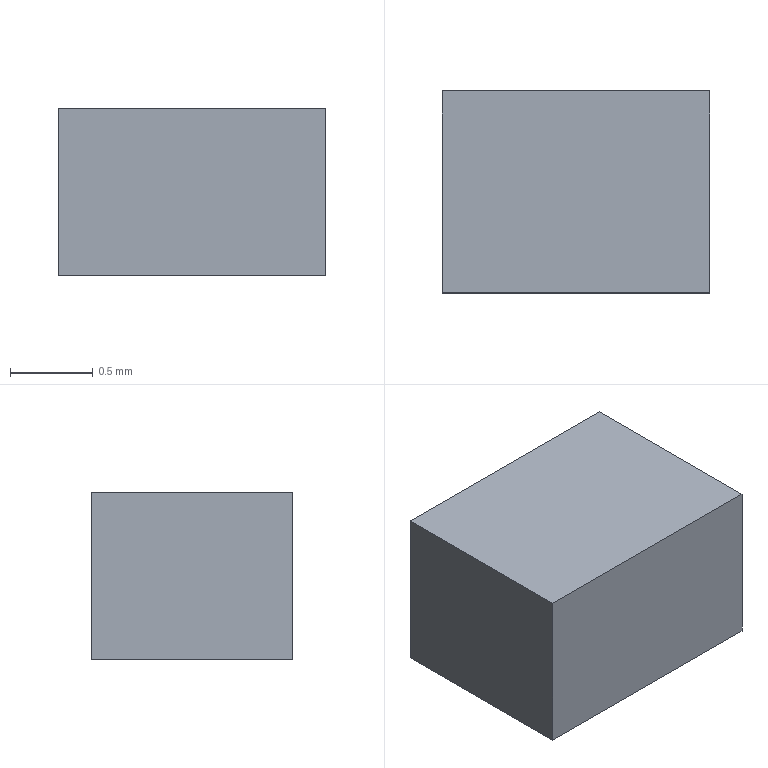Part | Creo | 1 solid | 6 faces | box 1.616 x 1.219 x 1.012 mm | volume 1.993 mm3 | plane 6
STEP:
#1=CARTESIAN_POINT('',(0.,0.,0.));
#2=DIRECTION('',(0.,0.,1.));
#3=DIRECTION('',(1.,0.,0.));
#4=AXIS2_PLACEMENT_3D('',#1,#2,#3);
#5=CARTESIAN_POINT('',(-0.8405,-0.644,0.));
#6=VERTEX_POINT('',#5);
#7=CARTESIAN_POINT('',(0.775,-0.644,0.));
#8=VERTEX_POINT('',#7);
#9=CARTESIAN_POINT('',(-0.8405,-0.644,0.));
#10=DIRECTION('',(1.,0.,0.));
#11=VECTOR('',#10,1.616);
#12=LINE('',#9,#11);
#13=EDGE_CURVE('',#6,#8,#12,.T.);
#14=ORIENTED_EDGE('',*,*,#13,.T.);
#15=CARTESIAN_POINT('',(0.775,0.575,0.));
#16=VERTEX_POINT('',#15);
#17=CARTESIAN_POINT('',(0.775,-0.644,0.));
#18=DIRECTION('',(0.,1.,0.));
#19=VECTOR('',#18,1.219);
#20=LINE('',#17,#19);
#21=EDGE_CURVE('',#8,#16,#20,.T.);
#22=ORIENTED_EDGE('',*,*,#21,.T.);
#23=CARTESIAN_POINT('',(-0.8405,0.575,0.));
#24=VERTEX_POINT('',#23);
#25=CARTESIAN_POINT('',(0.775,0.575,0.));
#26=DIRECTION('',(-1.,0.,0.));
#27=VECTOR('',#26,1.616);
#28=LINE('',#25,#27);
#29=EDGE_CURVE('',#16,#24,#28,.T.);
#30=ORIENTED_EDGE('',*,*,#29,.T.);
#31=CARTESIAN_POINT('',(-0.8405,0.575,0.));
#32=DIRECTION('',(0.,-1.,0.));
#33=VECTOR('',#32,1.219);
#34=LINE('',#31,#33);
#35=EDGE_CURVE('',#24,#6,#34,.T.);
#36=ORIENTED_EDGE('',*,*,#35,.T.);
#37=EDGE_LOOP('',(#14,#22,#30,#36));
#38=FACE_OUTER_BOUND('',#37,.F.);
#39=CARTESIAN_POINT('',(0.,0.,0.));
#40=DIRECTION('',(0.,0.,1.));
#41=DIRECTION('',(1.,0.,0.));
#42=AXIS2_PLACEMENT_3D('',#39,#40,#41);
#43=PLANE('',#42);
#44=ADVANCED_FACE('',(#38),#43,.F.);
#45=ORIENTED_EDGE('',*,*,#13,.F.);
#46=CARTESIAN_POINT('',(-0.8405,-0.644,1.012));
#47=VERTEX_POINT('',#46);
#48=CARTESIAN_POINT('',(-0.8405,-0.644,0.));
#49=DIRECTION('',(0.,0.,1.));
#50=VECTOR('',#49,1.012);
#51=LINE('',#48,#50);
#52=EDGE_CURVE('',#6,#47,#51,.T.);
#53=ORIENTED_EDGE('',*,*,#52,.T.);
#54=CARTESIAN_POINT('',(0.775,-0.644,1.012));
#55=VERTEX_POINT('',#54);
#56=CARTESIAN_POINT('',(-0.8405,-0.644,1.012));
#57=DIRECTION('',(1.,0.,0.));
#58=VECTOR('',#57,1.616);
#59=LINE('',#56,#58);
#60=EDGE_CURVE('',#47,#55,#59,.T.);
#61=ORIENTED_EDGE('',*,*,#60,.T.);
#62=CARTESIAN_POINT('',(0.775,-0.644,0.));
#63=DIRECTION('',(0.,0.,1.));
#64=VECTOR('',#63,1.012);
#65=LINE('',#62,#64);
#66=EDGE_CURVE('',#8,#55,#65,.T.);
#67=ORIENTED_EDGE('',*,*,#66,.F.);
#68=EDGE_LOOP('',(#45,#53,#61,#67));
#69=FACE_OUTER_BOUND('',#68,.F.);
#70=CARTESIAN_POINT('',(-0.8405,-0.644,0.));
#71=DIRECTION('',(0.,-1.,0.));
#72=DIRECTION('',(1.,0.,0.));
#73=AXIS2_PLACEMENT_3D('',#70,#71,#72);
#74=PLANE('',#73);
#75=ADVANCED_FACE('',(#69),#74,.T.);
#76=ORIENTED_EDGE('',*,*,#35,.F.);
#77=CARTESIAN_POINT('',(-0.8405,0.575,1.012));
#78=VERTEX_POINT('',#77);
#79=CARTESIAN_POINT('',(-0.8405,0.575,0.));
#80=DIRECTION('',(0.,0.,1.));
#81=VECTOR('',#80,1.012);
#82=LINE('',#79,#81);
#83=EDGE_CURVE('',#24,#78,#82,.T.);
#84=ORIENTED_EDGE('',*,*,#83,.T.);
#85=CARTESIAN_POINT('',(-0.8405,0.575,1.012));
#86=DIRECTION('',(0.,-1.,0.));
#87=VECTOR('',#86,1.219);
#88=LINE('',#85,#87);
#89=EDGE_CURVE('',#78,#47,#88,.T.);
#90=ORIENTED_EDGE('',*,*,#89,.T.);
#91=ORIENTED_EDGE('',*,*,#52,.F.);
#92=EDGE_LOOP('',(#76,#84,#90,#91));
#93=FACE_OUTER_BOUND('',#92,.F.);
#94=CARTESIAN_POINT('',(-0.8405,0.575,0.));
#95=DIRECTION('',(-1.,0.,0.));
#96=DIRECTION('',(0.,-1.,0.));
#97=AXIS2_PLACEMENT_3D('',#94,#95,#96);
#98=PLANE('',#97);
#99=ADVANCED_FACE('',(#93),#98,.T.);
#100=ORIENTED_EDGE('',*,*,#29,.F.);
#101=CARTESIAN_POINT('',(0.775,0.575,1.012));
#102=VERTEX_POINT('',#101);
#103=CARTESIAN_POINT('',(0.775,0.575,0.));
#104=DIRECTION('',(0.,0.,1.));
#105=VECTOR('',#104,1.012);
#106=LINE('',#103,#105);
#107=EDGE_CURVE('',#16,#102,#106,.T.);
#108=ORIENTED_EDGE('',*,*,#107,.T.);
#109=CARTESIAN_POINT('',(0.775,0.575,1.012));
#110=DIRECTION('',(-1.,0.,0.));
#111=VECTOR('',#110,1.616);
#112=LINE('',#109,#111);
#113=EDGE_CURVE('',#102,#78,#112,.T.);
#114=ORIENTED_EDGE('',*,*,#113,.T.);
#115=ORIENTED_EDGE('',*,*,#83,.F.);
#116=EDGE_LOOP('',(#100,#108,#114,#115));
#117=FACE_OUTER_BOUND('',#116,.F.);
#118=CARTESIAN_POINT('',(0.775,0.575,0.));
#119=DIRECTION('',(0.,1.,0.));
#120=DIRECTION('',(-1.,0.,0.));
#121=AXIS2_PLACEMENT_3D('',#118,#119,#120);
#122=PLANE('',#121);
#123=ADVANCED_FACE('',(#117),#122,.T.);
#124=ORIENTED_EDGE('',*,*,#21,.F.);
#125=ORIENTED_EDGE('',*,*,#66,.T.);
#126=CARTESIAN_POINT('',(0.775,-0.644,1.012));
#127=DIRECTION('',(0.,1.,0.));
#128=VECTOR('',#127,1.219);
#129=LINE('',#126,#128);
#130=EDGE_CURVE('',#55,#102,#129,.T.);
#131=ORIENTED_EDGE('',*,*,#130,.T.);
#132=ORIENTED_EDGE('',*,*,#107,.F.);
#133=EDGE_LOOP('',(#124,#125,#131,#132));
#134=FACE_OUTER_BOUND('',#133,.F.);
#135=CARTESIAN_POINT('',(0.775,-0.644,0.));
#136=DIRECTION('',(1.,0.,0.));
#137=DIRECTION('',(0.,1.,0.));
#138=AXIS2_PLACEMENT_3D('',#135,#136,#137);
#139=PLANE('',#138);
#140=ADVANCED_FACE('',(#134),#139,.T.);
#141=ORIENTED_EDGE('',*,*,#60,.F.);
#142=ORIENTED_EDGE('',*,*,#89,.F.);
#143=ORIENTED_EDGE('',*,*,#113,.F.);
#144=ORIENTED_EDGE('',*,*,#130,.F.);
#145=EDGE_LOOP('',(#141,#142,#143,#144));
#146=FACE_OUTER_BOUND('',#145,.F.);
#147=CARTESIAN_POINT('',(0.,0.,1.012));
#148=DIRECTION('',(0.,0.,1.));
#149=DIRECTION('',(1.,0.,0.));
#150=AXIS2_PLACEMENT_3D('',#147,#148,#149);
#151=PLANE('',#150);
#152=ADVANCED_FACE('',(#146),#151,.T.);
#153=CLOSED_SHELL('',(#44,#75,#99,#123,#140,#152));
#154=MANIFOLD_SOLID_BREP('',#153);
#155=(LENGTH_UNIT()NAMED_UNIT(*)SI_UNIT(.MILLI.,.METRE.));
#156=UNCERTAINTY_MEASURE_WITH_UNIT(LENGTH_MEASURE(0.0002263),#155,'','');
#157=(NAMED_UNIT(*)PLANE_ANGLE_UNIT()SI_UNIT($,.RADIAN.));
#158=PLANE_ANGLE_MEASURE_WITH_UNIT(PLANE_ANGLE_MEASURE(0.01745),#157);
#159=(CONVERSION_BASED_UNIT('DEGREE',#158)NAMED_UNIT(*)PLANE_ANGLE_UNIT());
#160=(NAMED_UNIT(*)SI_UNIT($,.STERADIAN.)SOLID_ANGLE_UNIT());
#161=(GEOMETRIC_REPRESENTATION_CONTEXT(3)GLOBAL_UNCERTAINTY_ASSIGNED_CONTEXT((#156))GLOBAL_UNIT_ASSIGNED_CONTEXT((#155,#159,#160))REPRESENTATION_CONTEXT('',''));
#162=ADVANCED_BREP_SHAPE_REPRESENTATION('',(#4,#154),#161);